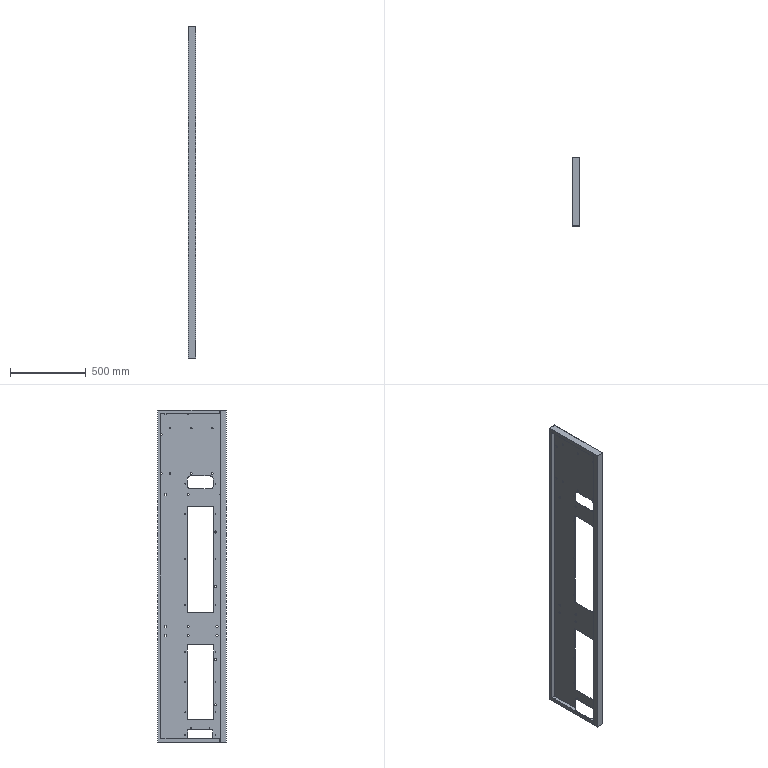Part | SolidWorks | features BaseBody 1 | 1 solid | 209 faces | box 50 x 450 x 2190 mm | volume 2821618 mm3 | plane 155 | cylinder 54 | commonest cylinder face diameters 6.5 x32 14 x8 11 x6 4.4 x4 40 x4